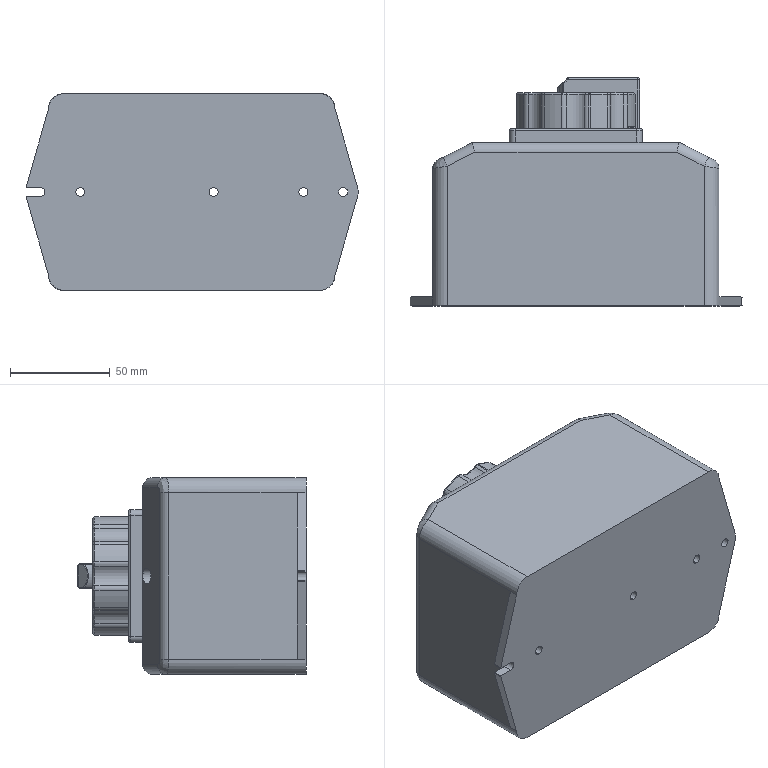Part | SolidWorks | features ICE 14, Fillet 11, HoleWzd 2, CirPattern 1, Extrusion 1 | 1 solid | 474 faces | box 166.689 x 114.5 x 98.75 mm | volume 1199464 mm3 | plane 211 | spline 128 | cylinder 92 | torus 41 | sphere 2 | commonest cylinder face diameters 6 x22 15 x12 2 x11 4.5 x9 10 x8 61 x8